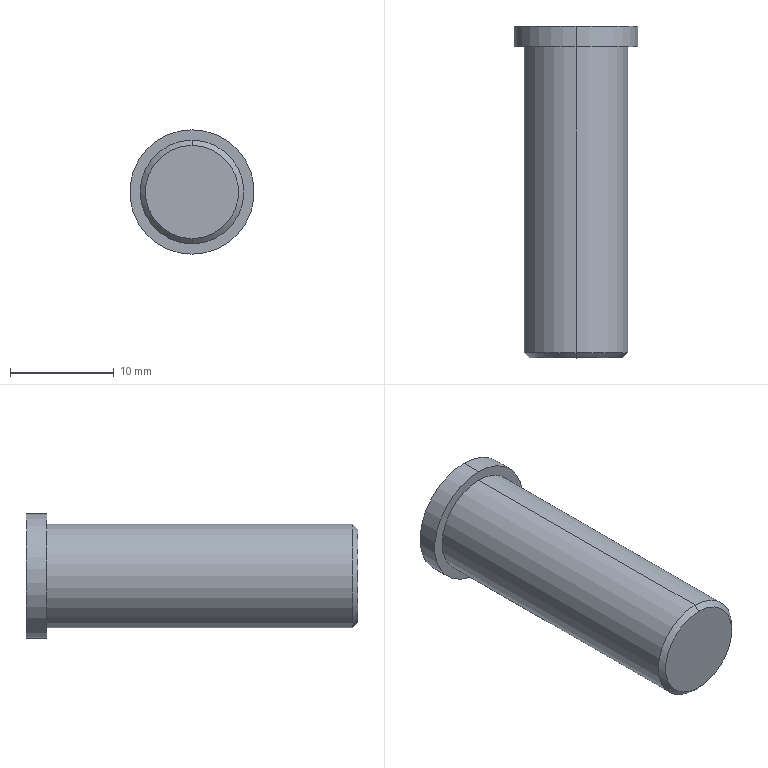Part | STEP file | BCC3 H12_11 | 1 solid | 9 faces | box 12 x 32 x 12 mm | volume 2579 mm3 | cylinder 4 | plane 3 | cone 2 | commonest cylinder face diameters 10 x2 12 x2
STEP:
#1=CARTESIAN_POINT('',(0.,0.,0.));
#2=DIRECTION('',(0.,0.,1.));
#3=DIRECTION('',(1.,0.,0.));
#4=AXIS2_PLACEMENT_3D('',#1,#2,#3);
#5=CARTESIAN_POINT('',(0.,0.,-4.5));
#6=VERTEX_POINT('',#5);
#7=CARTESIAN_POINT('',(0.,0.,4.5));
#8=VERTEX_POINT('',#7);
#9=CARTESIAN_POINT('',(0.,0.,0.));
#10=DIRECTION('',(0.,-1.,0.));
#11=DIRECTION('',(0.,0.,1.));
#12=AXIS2_PLACEMENT_3D('',#9,#10,#11);
#13=CIRCLE('',#12,4.5);
#14=CARTESIAN_POINT('',(0.,0.5,0.));
#15=DIRECTION('',(0.,1.,0.));
#16=DIRECTION('',(0.,0.,1.));
#17=AXIS2_PLACEMENT_3D('',#14,#15,#16);
#18=CONICAL_SURFACE('',#17,5.,0.7854);
#19=CARTESIAN_POINT('',(6.283,-0.5));
#20=DIRECTION('',(-1.,0.));
#21=VECTOR('',#20,1.);
#22=LINE('',#19,#21);
#23=(GEOMETRIC_REPRESENTATION_CONTEXT(2)PARAMETRIC_REPRESENTATION_CONTEXT()REPRESENTATION_CONTEXT('',''));
#24=DEFINITIONAL_REPRESENTATION('',(#22),#23);
#25=PCURVE('',#18,#24);
#26=CARTESIAN_POINT('',(0.,0.,0.));
#27=DIRECTION('',(0.,1.,0.));
#28=DIRECTION('',(0.,0.,1.));
#29=AXIS2_PLACEMENT_3D('',#26,#27,#28);
#30=PLANE('',#29);
#31=CARTESIAN_POINT('',(4.5,0.));
#32=CARTESIAN_POINT('',(4.5,-7.794));
#33=CARTESIAN_POINT('',(-2.25,-3.897));
#34=CARTESIAN_POINT('',(-9.,0.));
#35=CARTESIAN_POINT('',(-2.25,3.897));
#36=CARTESIAN_POINT('',(4.5,7.794));
#37=CARTESIAN_POINT('',(4.5,0.));
#38=(BOUNDED_CURVE()B_SPLINE_CURVE(2,(#31,#32,#33,#34,#35,#36,#37),.UNSPECIFIED.,.T.,.F.)B_SPLINE_CURVE_WITH_KNOTS((1,2,2,2,2,1),(-2.094,0.,2.094,4.189,6.283,8.378),.UNSPECIFIED.)CURVE()GEOMETRIC_REPRESENTATION_ITEM()RATIONAL_B_SPLINE_CURVE((1.,0.5,1.,0.5,1.,0.5,1.))REPRESENTATION_ITEM(''));
#39=(GEOMETRIC_REPRESENTATION_CONTEXT(2)PARAMETRIC_REPRESENTATION_CONTEXT()REPRESENTATION_CONTEXT('',''));
#40=DEFINITIONAL_REPRESENTATION('',(#38),#39);
#41=PCURVE('',#30,#40);
#42=SURFACE_CURVE('',#13,(#25,#41),.PCURVE_S1.);
#43=EDGE_CURVE('',#6,#8,#42,.T.);
#44=ORIENTED_EDGE('',*,*,#43,.F.);
#45=CARTESIAN_POINT('',(0.,0.5,-5.));
#46=VERTEX_POINT('',#45);
#47=CARTESIAN_POINT('',(0.,0.5,-5.));
#48=DIRECTION('',(0.,0.7071,-0.7071));
#49=VECTOR('',#48,1.);
#50=LINE('',#47,#49);
#51=CARTESIAN_POINT('',(3.142,0.));
#52=DIRECTION('',(0.,1.));
#53=VECTOR('',#52,1.);
#54=LINE('',#51,#53);
#55=(GEOMETRIC_REPRESENTATION_CONTEXT(2)PARAMETRIC_REPRESENTATION_CONTEXT()REPRESENTATION_CONTEXT('',''));
#56=DEFINITIONAL_REPRESENTATION('',(#54),#55);
#57=PCURVE('',#18,#56);
#58=CARTESIAN_POINT('',(0.,0.5,0.));
#59=DIRECTION('',(0.,1.,0.));
#60=DIRECTION('',(0.,0.,1.));
#61=AXIS2_PLACEMENT_3D('',#58,#59,#60);
#62=CONICAL_SURFACE('',#61,5.,0.7854);
#63=CARTESIAN_POINT('',(3.142,0.));
#64=DIRECTION('',(0.,1.));
#65=VECTOR('',#64,1.);
#66=LINE('',#63,#65);
#67=(GEOMETRIC_REPRESENTATION_CONTEXT(2)PARAMETRIC_REPRESENTATION_CONTEXT()REPRESENTATION_CONTEXT('',''));
#68=DEFINITIONAL_REPRESENTATION('',(#66),#67);
#69=PCURVE('',#62,#68);
#70=SURFACE_CURVE('',#50,(#57,#69),.PCURVE_S1.);
#71=EDGE_CURVE('',#6,#46,#70,.T.);
#72=ORIENTED_EDGE('',*,*,#71,.T.);
#73=CARTESIAN_POINT('',(0.,0.5,5.));
#74=VERTEX_POINT('',#73);
#75=CARTESIAN_POINT('',(0.,0.5,0.));
#76=DIRECTION('',(0.,1.,0.));
#77=DIRECTION('',(0.,0.,1.));
#78=AXIS2_PLACEMENT_3D('',#75,#76,#77);
#79=CIRCLE('',#78,5.);
#80=CARTESIAN_POINT('',(0.,0.));
#81=DIRECTION('',(1.,0.));
#82=VECTOR('',#81,1.);
#83=LINE('',#80,#82);
#84=(GEOMETRIC_REPRESENTATION_CONTEXT(2)PARAMETRIC_REPRESENTATION_CONTEXT()REPRESENTATION_CONTEXT('',''));
#85=DEFINITIONAL_REPRESENTATION('',(#83),#84);
#86=PCURVE('',#18,#85);
#87=CARTESIAN_POINT('',(0.,30.,0.));
#88=DIRECTION('',(0.,-1.,0.));
#89=DIRECTION('',(0.,0.,-1.));
#90=AXIS2_PLACEMENT_3D('',#87,#88,#89);
#91=CYLINDRICAL_SURFACE('',#90,5.);
#92=CARTESIAN_POINT('',(3.142,29.5));
#93=DIRECTION('',(-1.,0.));
#94=VECTOR('',#93,1.);
#95=LINE('',#92,#94);
#96=(GEOMETRIC_REPRESENTATION_CONTEXT(2)PARAMETRIC_REPRESENTATION_CONTEXT()REPRESENTATION_CONTEXT('',''));
#97=DEFINITIONAL_REPRESENTATION('',(#95),#96);
#98=PCURVE('',#91,#97);
#99=SURFACE_CURVE('',#79,(#86,#98),.PCURVE_S1.);
#100=EDGE_CURVE('',#74,#46,#99,.T.);
#101=ORIENTED_EDGE('',*,*,#100,.F.);
#102=CARTESIAN_POINT('',(0.,0.5,5.));
#103=DIRECTION('',(0.,0.7071,0.7071));
#104=VECTOR('',#103,1.);
#105=LINE('',#102,#104);
#106=CARTESIAN_POINT('',(0.,0.));
#107=DIRECTION('',(0.,1.));
#108=VECTOR('',#107,1.);
#109=LINE('',#106,#108);
#110=(GEOMETRIC_REPRESENTATION_CONTEXT(2)PARAMETRIC_REPRESENTATION_CONTEXT()REPRESENTATION_CONTEXT('',''));
#111=DEFINITIONAL_REPRESENTATION('',(#109),#110);
#112=PCURVE('',#18,#111);
#113=CARTESIAN_POINT('',(6.283,0.));
#114=DIRECTION('',(0.,1.));
#115=VECTOR('',#114,1.);
#116=LINE('',#113,#115);
#117=(GEOMETRIC_REPRESENTATION_CONTEXT(2)PARAMETRIC_REPRESENTATION_CONTEXT()REPRESENTATION_CONTEXT('',''));
#118=DEFINITIONAL_REPRESENTATION('',(#116),#117);
#119=PCURVE('',#62,#118);
#120=SURFACE_CURVE('',#105,(#112,#119),.PCURVE_S1.);
#121=EDGE_CURVE('',#8,#74,#120,.T.);
#122=ORIENTED_EDGE('',*,*,#121,.F.);
#123=EDGE_LOOP('',(#44,#72,#101,#122));
#124=FACE_BOUND('',#123,.T.);
#125=ADVANCED_FACE('',(#124),#18,.T.);
#126=CARTESIAN_POINT('',(0.,32.,6.));
#127=VERTEX_POINT('',#126);
#128=CARTESIAN_POINT('',(0.,32.,-6.));
#129=VERTEX_POINT('',#128);
#130=CARTESIAN_POINT('',(0.,32.,0.));
#131=DIRECTION('',(0.,1.,0.));
#132=DIRECTION('',(0.,0.,1.));
#133=AXIS2_PLACEMENT_3D('',#130,#131,#132);
#134=CIRCLE('',#133,6.);
#135=CARTESIAN_POINT('',(0.,32.,0.));
#136=DIRECTION('',(0.,-1.,0.));
#137=DIRECTION('',(0.,0.,-1.));
#138=AXIS2_PLACEMENT_3D('',#135,#136,#137);
#139=CYLINDRICAL_SURFACE('',#138,6.);
#140=CARTESIAN_POINT('',(3.142,0.));
#141=DIRECTION('',(-1.,0.));
#142=VECTOR('',#141,1.);
#143=LINE('',#140,#142);
#144=(GEOMETRIC_REPRESENTATION_CONTEXT(2)PARAMETRIC_REPRESENTATION_CONTEXT()REPRESENTATION_CONTEXT('',''));
#145=DEFINITIONAL_REPRESENTATION('',(#143),#144);
#146=PCURVE('',#139,#145);
#147=CARTESIAN_POINT('',(0.,32.,0.));
#148=DIRECTION('',(0.,1.,0.));
#149=DIRECTION('',(0.,0.,1.));
#150=AXIS2_PLACEMENT_3D('',#147,#148,#149);
#151=PLANE('',#150);
#152=CARTESIAN_POINT('',(0.,0.));
#153=DIRECTION('',(1.,0.));
#154=AXIS2_PLACEMENT_2D('',#152,#153);
#155=CIRCLE('',#154,6.);
#156=(GEOMETRIC_REPRESENTATION_CONTEXT(2)PARAMETRIC_REPRESENTATION_CONTEXT()REPRESENTATION_CONTEXT('',''));
#157=DEFINITIONAL_REPRESENTATION('',(#155),#156);
#158=PCURVE('',#151,#157);
#159=SURFACE_CURVE('',#134,(#146,#158),.PCURVE_S1.);
#160=EDGE_CURVE('',#127,#129,#159,.T.);
#161=ORIENTED_EDGE('',*,*,#160,.F.);
#162=CARTESIAN_POINT('',(0.,30.,6.));
#163=VERTEX_POINT('',#162);
#164=CARTESIAN_POINT('',(0.,32.,6.));
#165=DIRECTION('',(0.,-1.,0.));
#166=VECTOR('',#165,1.);
#167=LINE('',#164,#166);
#168=CARTESIAN_POINT('',(3.142,0.));
#169=DIRECTION('',(0.,1.));
#170=VECTOR('',#169,1.);
#171=LINE('',#168,#170);
#172=(GEOMETRIC_REPRESENTATION_CONTEXT(2)PARAMETRIC_REPRESENTATION_CONTEXT()REPRESENTATION_CONTEXT('',''));
#173=DEFINITIONAL_REPRESENTATION('',(#171),#172);
#174=PCURVE('',#139,#173);
#175=CARTESIAN_POINT('',(0.,32.,0.));
#176=DIRECTION('',(0.,-1.,0.));
#177=DIRECTION('',(0.,0.,-1.));
#178=AXIS2_PLACEMENT_3D('',#175,#176,#177);
#179=CYLINDRICAL_SURFACE('',#178,6.);
#180=CARTESIAN_POINT('',(3.142,0.));
#181=DIRECTION('',(0.,1.));
#182=VECTOR('',#181,1.);
#183=LINE('',#180,#182);
#184=(GEOMETRIC_REPRESENTATION_CONTEXT(2)PARAMETRIC_REPRESENTATION_CONTEXT()REPRESENTATION_CONTEXT('',''));
#185=DEFINITIONAL_REPRESENTATION('',(#183),#184);
#186=PCURVE('',#179,#185);
#187=SURFACE_CURVE('',#167,(#174,#186),.PCURVE_S1.);
#188=EDGE_CURVE('',#127,#163,#187,.T.);
#189=ORIENTED_EDGE('',*,*,#188,.T.);
#190=CARTESIAN_POINT('',(0.,30.,-6.));
#191=VERTEX_POINT('',#190);
#192=CARTESIAN_POINT('',(0.,30.,0.));
#193=DIRECTION('',(0.,1.,0.));
#194=DIRECTION('',(0.,0.,1.));
#195=AXIS2_PLACEMENT_3D('',#192,#193,#194);
#196=CIRCLE('',#195,6.);
#197=CARTESIAN_POINT('',(3.142,2.));
#198=DIRECTION('',(-1.,0.));
#199=VECTOR('',#198,1.);
#200=LINE('',#197,#199);
#201=(GEOMETRIC_REPRESENTATION_CONTEXT(2)PARAMETRIC_REPRESENTATION_CONTEXT()REPRESENTATION_CONTEXT('',''));
#202=DEFINITIONAL_REPRESENTATION('',(#200),#201);
#203=PCURVE('',#139,#202);
#204=CARTESIAN_POINT('',(0.,30.,0.));
#205=DIRECTION('',(0.,1.,0.));
#206=DIRECTION('',(0.,0.,1.));
#207=AXIS2_PLACEMENT_3D('',#204,#205,#206);
#208=PLANE('',#207);
#209=CARTESIAN_POINT('',(0.,0.));
#210=DIRECTION('',(1.,0.));
#211=AXIS2_PLACEMENT_2D('',#209,#210);
#212=CIRCLE('',#211,6.);
#213=(GEOMETRIC_REPRESENTATION_CONTEXT(2)PARAMETRIC_REPRESENTATION_CONTEXT()REPRESENTATION_CONTEXT('',''));
#214=DEFINITIONAL_REPRESENTATION('',(#212),#213);
#215=PCURVE('',#208,#214);
#216=SURFACE_CURVE('',#196,(#203,#215),.PCURVE_S1.);
#217=EDGE_CURVE('',#163,#191,#216,.T.);
#218=ORIENTED_EDGE('',*,*,#217,.T.);
#219=CARTESIAN_POINT('',(0.,32.,-6.));
#220=DIRECTION('',(0.,-1.,0.));
#221=VECTOR('',#220,1.);
#222=LINE('',#219,#221);
#223=CARTESIAN_POINT('',(0.,0.));
#224=DIRECTION('',(0.,1.));
#225=VECTOR('',#224,1.);
#226=LINE('',#223,#225);
#227=(GEOMETRIC_REPRESENTATION_CONTEXT(2)PARAMETRIC_REPRESENTATION_CONTEXT()REPRESENTATION_CONTEXT('',''));
#228=DEFINITIONAL_REPRESENTATION('',(#226),#227);
#229=PCURVE('',#139,#228);
#230=CARTESIAN_POINT('',(6.283,0.));
#231=DIRECTION('',(0.,1.));
#232=VECTOR('',#231,1.);
#233=LINE('',#230,#232);
#234=(GEOMETRIC_REPRESENTATION_CONTEXT(2)PARAMETRIC_REPRESENTATION_CONTEXT()REPRESENTATION_CONTEXT('',''));
#235=DEFINITIONAL_REPRESENTATION('',(#233),#234);
#236=PCURVE('',#179,#235);
#237=SURFACE_CURVE('',#222,(#229,#236),.PCURVE_S1.);
#238=EDGE_CURVE('',#129,#191,#237,.T.);
#239=ORIENTED_EDGE('',*,*,#238,.F.);
#240=EDGE_LOOP('',(#161,#189,#218,#239));
#241=FACE_BOUND('',#240,.T.);
#242=ADVANCED_FACE('',(#241),#139,.T.);
#243=CARTESIAN_POINT('',(0.,30.,5.));
#244=VERTEX_POINT('',#243);
#245=CARTESIAN_POINT('',(0.,30.,-5.));
#246=VERTEX_POINT('',#245);
#247=CARTESIAN_POINT('',(0.,30.,0.));
#248=DIRECTION('',(0.,1.,0.));
#249=DIRECTION('',(0.,0.,1.));
#250=AXIS2_PLACEMENT_3D('',#247,#248,#249);
#251=CIRCLE('',#250,5.);
#252=CARTESIAN_POINT('',(3.142,0.));
#253=DIRECTION('',(-1.,0.));
#254=VECTOR('',#253,1.);
#255=LINE('',#252,#254);
#256=(GEOMETRIC_REPRESENTATION_CONTEXT(2)PARAMETRIC_REPRESENTATION_CONTEXT()REPRESENTATION_CONTEXT('',''));
#257=DEFINITIONAL_REPRESENTATION('',(#255),#256);
#258=PCURVE('',#91,#257);
#259=CARTESIAN_POINT('',(0.,0.));
#260=DIRECTION('',(1.,0.));
#261=AXIS2_PLACEMENT_2D('',#259,#260);
#262=CIRCLE('',#261,5.);
#263=(GEOMETRIC_REPRESENTATION_CONTEXT(2)PARAMETRIC_REPRESENTATION_CONTEXT()REPRESENTATION_CONTEXT('',''));
#264=DEFINITIONAL_REPRESENTATION('',(#262),#263);
#265=PCURVE('',#208,#264);
#266=SURFACE_CURVE('',#251,(#258,#265),.PCURVE_S1.);
#267=EDGE_CURVE('',#244,#246,#266,.T.);
#268=ORIENTED_EDGE('',*,*,#267,.F.);
#269=CARTESIAN_POINT('',(0.,30.,5.));
#270=DIRECTION('',(0.,-1.,0.));
#271=VECTOR('',#270,1.);
#272=LINE('',#269,#271);
#273=CARTESIAN_POINT('',(3.142,0.));
#274=DIRECTION('',(0.,1.));
#275=VECTOR('',#274,1.);
#276=LINE('',#273,#275);
#277=(GEOMETRIC_REPRESENTATION_CONTEXT(2)PARAMETRIC_REPRESENTATION_CONTEXT()REPRESENTATION_CONTEXT('',''));
#278=DEFINITIONAL_REPRESENTATION('',(#276),#277);
#279=PCURVE('',#91,#278);
#280=CARTESIAN_POINT('',(0.,30.,0.));
#281=DIRECTION('',(0.,-1.,0.));
#282=DIRECTION('',(0.,0.,-1.));
#283=AXIS2_PLACEMENT_3D('',#280,#281,#282);
#284=CYLINDRICAL_SURFACE('',#283,5.);
#285=CARTESIAN_POINT('',(3.142,0.));
#286=DIRECTION('',(0.,1.));
#287=VECTOR('',#286,1.);
#288=LINE('',#285,#287);
#289=(GEOMETRIC_REPRESENTATION_CONTEXT(2)PARAMETRIC_REPRESENTATION_CONTEXT()REPRESENTATION_CONTEXT('',''));
#290=DEFINITIONAL_REPRESENTATION('',(#288),#289);
#291=PCURVE('',#284,#290);
#292=SURFACE_CURVE('',#272,(#279,#291),.PCURVE_S1.);
#293=EDGE_CURVE('',#244,#74,#292,.T.);
#294=ORIENTED_EDGE('',*,*,#293,.T.);
#295=ORIENTED_EDGE('',*,*,#100,.T.);
#296=CARTESIAN_POINT('',(0.,30.,-5.));
#297=DIRECTION('',(0.,-1.,0.));
#298=VECTOR('',#297,1.);
#299=LINE('',#296,#298);
#300=CARTESIAN_POINT('',(0.,0.));
#301=DIRECTION('',(0.,1.));
#302=VECTOR('',#301,1.);
#303=LINE('',#300,#302);
#304=(GEOMETRIC_REPRESENTATION_CONTEXT(2)PARAMETRIC_REPRESENTATION_CONTEXT()REPRESENTATION_CONTEXT('',''));
#305=DEFINITIONAL_REPRESENTATION('',(#303),#304);
#306=PCURVE('',#91,#305);
#307=CARTESIAN_POINT('',(6.283,0.));
#308=DIRECTION('',(0.,1.));
#309=VECTOR('',#308,1.);
#310=LINE('',#307,#309);
#311=(GEOMETRIC_REPRESENTATION_CONTEXT(2)PARAMETRIC_REPRESENTATION_CONTEXT()REPRESENTATION_CONTEXT('',''));
#312=DEFINITIONAL_REPRESENTATION('',(#310),#311);
#313=PCURVE('',#284,#312);
#314=SURFACE_CURVE('',#299,(#306,#313),.PCURVE_S1.);
#315=EDGE_CURVE('',#246,#46,#314,.T.);
#316=ORIENTED_EDGE('',*,*,#315,.F.);
#317=EDGE_LOOP('',(#268,#294,#295,#316));
#318=FACE_BOUND('',#317,.T.);
#319=ADVANCED_FACE('',(#318),#91,.T.);
#320=ORIENTED_EDGE('',*,*,#293,.F.);
#321=CARTESIAN_POINT('',(0.,30.,0.));
#322=DIRECTION('',(0.,1.,0.));
#323=DIRECTION('',(0.,0.,1.));
#324=AXIS2_PLACEMENT_3D('',#321,#322,#323);
#325=CIRCLE('',#324,5.);
#326=CARTESIAN_POINT('',(9.425,0.));
#327=DIRECTION('',(-1.,0.));
#328=VECTOR('',#327,1.);
#329=LINE('',#326,#328);
#330=(GEOMETRIC_REPRESENTATION_CONTEXT(2)PARAMETRIC_REPRESENTATION_CONTEXT()REPRESENTATION_CONTEXT('',''));
#331=DEFINITIONAL_REPRESENTATION('',(#329),#330);
#332=PCURVE('',#284,#331);
#333=CARTESIAN_POINT('',(0.,0.));
#334=DIRECTION('',(1.,0.));
#335=AXIS2_PLACEMENT_2D('',#333,#334);
#336=CIRCLE('',#335,5.);
#337=(GEOMETRIC_REPRESENTATION_CONTEXT(2)PARAMETRIC_REPRESENTATION_CONTEXT()REPRESENTATION_CONTEXT('',''));
#338=DEFINITIONAL_REPRESENTATION('',(#336),#337);
#339=PCURVE('',#208,#338);
#340=SURFACE_CURVE('',#325,(#332,#339),.PCURVE_S1.);
#341=EDGE_CURVE('',#246,#244,#340,.T.);
#342=ORIENTED_EDGE('',*,*,#341,.F.);
#343=ORIENTED_EDGE('',*,*,#315,.T.);
#344=CARTESIAN_POINT('',(0.,0.5,0.));
#345=DIRECTION('',(0.,1.,0.));
#346=DIRECTION('',(0.,0.,1.));
#347=AXIS2_PLACEMENT_3D('',#344,#345,#346);
#348=CIRCLE('',#347,5.);
#349=CARTESIAN_POINT('',(9.425,29.5));
#350=DIRECTION('',(-1.,0.));
#351=VECTOR('',#350,1.);
#352=LINE('',#349,#351);
#353=(GEOMETRIC_REPRESENTATION_CONTEXT(2)PARAMETRIC_REPRESENTATION_CONTEXT()REPRESENTATION_CONTEXT('',''));
#354=DEFINITIONAL_REPRESENTATION('',(#352),#353);
#355=PCURVE('',#284,#354);
#356=CARTESIAN_POINT('',(0.,0.));
#357=DIRECTION('',(1.,0.));
#358=VECTOR('',#357,1.);
#359=LINE('',#356,#358);
#360=(GEOMETRIC_REPRESENTATION_CONTEXT(2)PARAMETRIC_REPRESENTATION_CONTEXT()REPRESENTATION_CONTEXT('',''));
#361=DEFINITIONAL_REPRESENTATION('',(#359),#360);
#362=PCURVE('',#62,#361);
#363=SURFACE_CURVE('',#348,(#355,#362),.PCURVE_S1.);
#364=EDGE_CURVE('',#46,#74,#363,.T.);
#365=ORIENTED_EDGE('',*,*,#364,.T.);
#366=EDGE_LOOP('',(#320,#342,#343,#365));
#367=FACE_BOUND('',#366,.T.);
#368=ADVANCED_FACE('',(#367),#284,.T.);
#369=CARTESIAN_POINT('',(0.,0.,0.));
#370=DIRECTION('',(0.,-1.,0.));
#371=DIRECTION('',(0.,0.,1.));
#372=AXIS2_PLACEMENT_3D('',#369,#370,#371);
#373=CIRCLE('',#372,4.5);
#374=CARTESIAN_POINT('',(4.5,0.));
#375=CARTESIAN_POINT('',(4.5,-7.794));
#376=CARTESIAN_POINT('',(-2.25,-3.897));
#377=CARTESIAN_POINT('',(-9.,0.));
#378=CARTESIAN_POINT('',(-2.25,3.897));
#379=CARTESIAN_POINT('',(4.5,7.794));
#380=CARTESIAN_POINT('',(4.5,0.));
#381=(BOUNDED_CURVE()B_SPLINE_CURVE(2,(#374,#375,#376,#377,#378,#379,#380),.UNSPECIFIED.,.T.,.F.)B_SPLINE_CURVE_WITH_KNOTS((1,2,2,2,2,1),(-2.094,0.,2.094,4.189,6.283,8.378),.UNSPECIFIED.)CURVE()GEOMETRIC_REPRESENTATION_ITEM()RATIONAL_B_SPLINE_CURVE((1.,0.5,1.,0.5,1.,0.5,1.))REPRESENTATION_ITEM(''));
#382=(GEOMETRIC_REPRESENTATION_CONTEXT(2)PARAMETRIC_REPRESENTATION_CONTEXT()REPRESENTATION_CONTEXT('',''));
#383=DEFINITIONAL_REPRESENTATION('',(#381),#382);
#384=PCURVE('',#30,#383);
#385=CARTESIAN_POINT('',(6.283,-0.5));
#386=DIRECTION('',(-1.,0.));
#387=VECTOR('',#386,1.);
#388=LINE('',#385,#387);
#389=(GEOMETRIC_REPRESENTATION_CONTEXT(2)PARAMETRIC_REPRESENTATION_CONTEXT()REPRESENTATION_CONTEXT('',''));
#390=DEFINITIONAL_REPRESENTATION('',(#388),#389);
#391=PCURVE('',#62,#390);
#392=SURFACE_CURVE('',#373,(#384,#391),.PCURVE_S1.);
#393=EDGE_CURVE('',#8,#6,#392,.T.);
#394=ORIENTED_EDGE('',*,*,#393,.T.);
#395=ORIENTED_EDGE('',*,*,#43,.T.);
#396=EDGE_LOOP('',(#394,#395));
#397=FACE_BOUND('',#396,.T.);
#398=ADVANCED_FACE('',(#397),#30,.F.);
#399=CARTESIAN_POINT('',(0.,30.,0.));
#400=DIRECTION('',(0.,1.,0.));
#401=DIRECTION('',(0.,0.,1.));
#402=AXIS2_PLACEMENT_3D('',#399,#400,#401);
#403=CIRCLE('',#402,6.);
#404=CARTESIAN_POINT('',(0.,0.));
#405=DIRECTION('',(1.,0.));
#406=AXIS2_PLACEMENT_2D('',#404,#405);
#407=CIRCLE('',#406,6.);
#408=(GEOMETRIC_REPRESENTATION_CONTEXT(2)PARAMETRIC_REPRESENTATION_CONTEXT()REPRESENTATION_CONTEXT('',''));
#409=DEFINITIONAL_REPRESENTATION('',(#407),#408);
#410=PCURVE('',#208,#409);
#411=CARTESIAN_POINT('',(9.425,2.));
#412=DIRECTION('',(-1.,0.));
#413=VECTOR('',#412,1.);
#414=LINE('',#411,#413);
#415=(GEOMETRIC_REPRESENTATION_CONTEXT(2)PARAMETRIC_REPRESENTATION_CONTEXT()REPRESENTATION_CONTEXT('',''));
#416=DEFINITIONAL_REPRESENTATION('',(#414),#415);
#417=PCURVE('',#179,#416);
#418=SURFACE_CURVE('',#403,(#410,#417),.PCURVE_S1.);
#419=EDGE_CURVE('',#191,#163,#418,.T.);
#420=ORIENTED_EDGE('',*,*,#419,.F.);
#421=ORIENTED_EDGE('',*,*,#217,.F.);
#422=EDGE_LOOP('',(#420,#421));
#423=FACE_BOUND('',#422,.T.);
#424=ORIENTED_EDGE('',*,*,#341,.T.);
#425=ORIENTED_EDGE('',*,*,#267,.T.);
#426=EDGE_LOOP('',(#424,#425));
#427=FACE_BOUND('',#426,.T.);
#428=ADVANCED_FACE('',(#423,#427),#208,.F.);
#429=ORIENTED_EDGE('',*,*,#188,.F.);
#430=CARTESIAN_POINT('',(0.,32.,0.));
#431=DIRECTION('',(0.,1.,0.));
#432=DIRECTION('',(0.,0.,1.));
#433=AXIS2_PLACEMENT_3D('',#430,#431,#432);
#434=CIRCLE('',#433,6.);
#435=CARTESIAN_POINT('',(9.425,0.));
#436=DIRECTION('',(-1.,0.));
#437=VECTOR('',#436,1.);
#438=LINE('',#435,#437);
#439=(GEOMETRIC_REPRESENTATION_CONTEXT(2)PARAMETRIC_REPRESENTATION_CONTEXT()REPRESENTATION_CONTEXT('',''));
#440=DEFINITIONAL_REPRESENTATION('',(#438),#439);
#441=PCURVE('',#179,#440);
#442=CARTESIAN_POINT('',(0.,0.));
#443=DIRECTION('',(1.,0.));
#444=AXIS2_PLACEMENT_2D('',#442,#443);
#445=CIRCLE('',#444,6.);
#446=(GEOMETRIC_REPRESENTATION_CONTEXT(2)PARAMETRIC_REPRESENTATION_CONTEXT()REPRESENTATION_CONTEXT('',''));
#447=DEFINITIONAL_REPRESENTATION('',(#445),#446);
#448=PCURVE('',#151,#447);
#449=SURFACE_CURVE('',#434,(#441,#448),.PCURVE_S1.);
#450=EDGE_CURVE('',#129,#127,#449,.T.);
#451=ORIENTED_EDGE('',*,*,#450,.F.);
#452=ORIENTED_EDGE('',*,*,#238,.T.);
#453=ORIENTED_EDGE('',*,*,#419,.T.);
#454=EDGE_LOOP('',(#429,#451,#452,#453));
#455=FACE_BOUND('',#454,.T.);
#456=ADVANCED_FACE('',(#455),#179,.T.);
#457=ORIENTED_EDGE('',*,*,#450,.T.);
#458=ORIENTED_EDGE('',*,*,#160,.T.);
#459=EDGE_LOOP('',(#457,#458));
#460=FACE_BOUND('',#459,.T.);
#461=ADVANCED_FACE('',(#460),#151,.T.);
#462=ORIENTED_EDGE('',*,*,#71,.F.);
#463=ORIENTED_EDGE('',*,*,#393,.F.);
#464=ORIENTED_EDGE('',*,*,#121,.T.);
#465=ORIENTED_EDGE('',*,*,#364,.F.);
#466=EDGE_LOOP('',(#462,#463,#464,#465));
#467=FACE_BOUND('',#466,.T.);
#468=ADVANCED_FACE('',(#467),#62,.T.);
#469=CLOSED_SHELL('',(#125,#242,#319,#368,#398,#428,#456,#461,#468));
#470=MANIFOLD_SOLID_BREP('',#469);
#471=(LENGTH_UNIT()NAMED_UNIT(*)SI_UNIT(.MILLI.,.METRE.));
#472=UNCERTAINTY_MEASURE_WITH_UNIT(LENGTH_MEASURE(0.0000001),#471,'','');
#473=(NAMED_UNIT(*)PLANE_ANGLE_UNIT()SI_UNIT($,.RADIAN.));
#474=(NAMED_UNIT(*)SI_UNIT($,.STERADIAN.)SOLID_ANGLE_UNIT());
#475=(GEOMETRIC_REPRESENTATION_CONTEXT(3)GLOBAL_UNCERTAINTY_ASSIGNED_CONTEXT((#472))GLOBAL_UNIT_ASSIGNED_CONTEXT((#471,#473,#474))REPRESENTATION_CONTEXT('',''));
#476=ADVANCED_BREP_SHAPE_REPRESENTATION('',(#4,#470),#475);